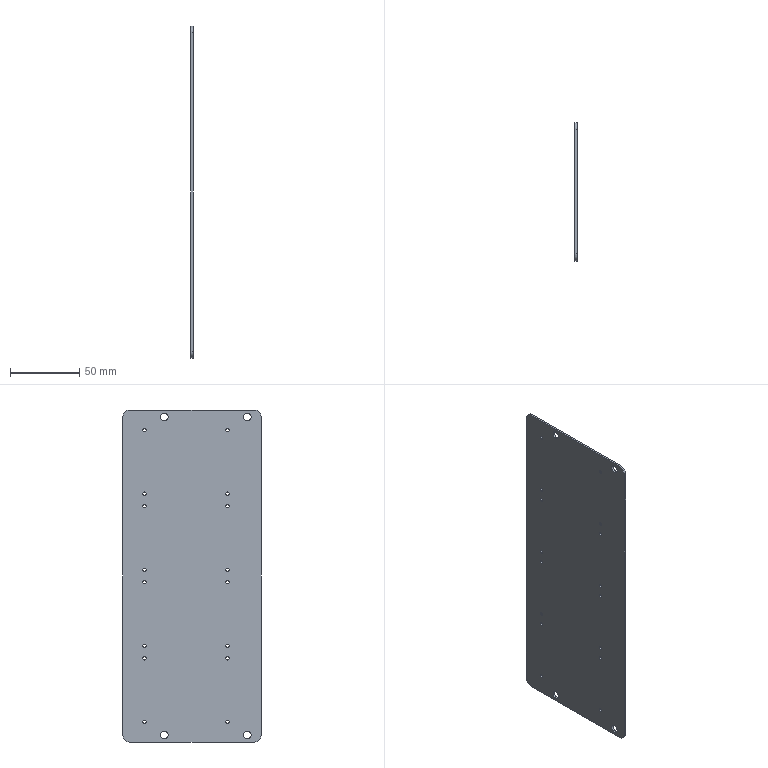Part | NX | features BREP 1 | 1 solid | 30 faces | box 1.5 x 100 x 240 mm | volume 35707 mm3 | cylinder 24 | plane 6 | commonest cylinder face diameters 2.5 x16 5.5 x4 10 x4
STEP:
#1=CARTESIAN_POINT('',(1.5,20.,-117.75));
#2=VERTEX_POINT('',#1);
#3=CARTESIAN_POINT('',(1.5,20.,-115.));
#4=DIRECTION('',(1.,0.,0.));
#5=DIRECTION('',(0.,0.,-1.));
#6=AXIS2_PLACEMENT_3D('',#3,#4,#5);
#7=CIRCLE('',#6,2.75);
#8=EDGE_CURVE('',#2,#2,#7,.T.);
#9=ORIENTED_EDGE('',*,*,#8,.T.);
#10=EDGE_LOOP('',(#9));
#11=FACE_BOUND('',#10,.T.);
#12=CARTESIAN_POINT('',(0.,20.,-117.75));
#13=VERTEX_POINT('',#12);
#14=CARTESIAN_POINT('',(0.,20.,-115.));
#15=DIRECTION('',(1.,0.,0.));
#16=DIRECTION('',(0.,0.,-1.));
#17=AXIS2_PLACEMENT_3D('',#14,#15,#16);
#18=CIRCLE('',#17,2.75);
#19=EDGE_CURVE('',#13,#13,#18,.T.);
#20=ORIENTED_EDGE('',*,*,#19,.F.);
#21=EDGE_LOOP('',(#20));
#22=FACE_BOUND('',#21,.T.);
#23=CARTESIAN_POINT('',(1.5,20.,-115.));
#24=DIRECTION('',(1.,0.,0.));
#25=DIRECTION('',(0.,0.,-1.));
#26=AXIS2_PLACEMENT_3D('',#23,#24,#25);
#27=CYLINDRICAL_SURFACE('',#26,2.75);
#28=ADVANCED_FACE('',(#11,#22),#27,.F.);
#29=CARTESIAN_POINT('',(1.5,-40.,-117.75));
#30=VERTEX_POINT('',#29);
#31=CARTESIAN_POINT('',(1.5,-40.,-115.));
#32=DIRECTION('',(1.,0.,0.));
#33=DIRECTION('',(0.,0.,-1.));
#34=AXIS2_PLACEMENT_3D('',#31,#32,#33);
#35=CIRCLE('',#34,2.75);
#36=EDGE_CURVE('',#30,#30,#35,.T.);
#37=ORIENTED_EDGE('',*,*,#36,.T.);
#38=EDGE_LOOP('',(#37));
#39=FACE_BOUND('',#38,.T.);
#40=CARTESIAN_POINT('',(0.,-40.,-117.75));
#41=VERTEX_POINT('',#40);
#42=CARTESIAN_POINT('',(0.,-40.,-115.));
#43=DIRECTION('',(1.,0.,0.));
#44=DIRECTION('',(0.,0.,-1.));
#45=AXIS2_PLACEMENT_3D('',#42,#43,#44);
#46=CIRCLE('',#45,2.75);
#47=EDGE_CURVE('',#41,#41,#46,.T.);
#48=ORIENTED_EDGE('',*,*,#47,.F.);
#49=EDGE_LOOP('',(#48));
#50=FACE_BOUND('',#49,.T.);
#51=CARTESIAN_POINT('',(1.5,-40.,-115.));
#52=DIRECTION('',(1.,0.,0.));
#53=DIRECTION('',(0.,0.,-1.));
#54=AXIS2_PLACEMENT_3D('',#51,#52,#53);
#55=CYLINDRICAL_SURFACE('',#54,2.75);
#56=ADVANCED_FACE('',(#39,#50),#55,.F.);
#57=CARTESIAN_POINT('',(1.5,20.,112.25));
#58=VERTEX_POINT('',#57);
#59=CARTESIAN_POINT('',(1.5,20.,115.));
#60=DIRECTION('',(1.,0.,0.));
#61=DIRECTION('',(0.,0.,-1.));
#62=AXIS2_PLACEMENT_3D('',#59,#60,#61);
#63=CIRCLE('',#62,2.75);
#64=EDGE_CURVE('',#58,#58,#63,.T.);
#65=ORIENTED_EDGE('',*,*,#64,.T.);
#66=EDGE_LOOP('',(#65));
#67=FACE_BOUND('',#66,.T.);
#68=CARTESIAN_POINT('',(0.,20.,112.25));
#69=VERTEX_POINT('',#68);
#70=CARTESIAN_POINT('',(0.,20.,115.));
#71=DIRECTION('',(1.,0.,0.));
#72=DIRECTION('',(0.,0.,-1.));
#73=AXIS2_PLACEMENT_3D('',#70,#71,#72);
#74=CIRCLE('',#73,2.75);
#75=EDGE_CURVE('',#69,#69,#74,.T.);
#76=ORIENTED_EDGE('',*,*,#75,.F.);
#77=EDGE_LOOP('',(#76));
#78=FACE_BOUND('',#77,.T.);
#79=CARTESIAN_POINT('',(1.5,20.,115.));
#80=DIRECTION('',(1.,0.,0.));
#81=DIRECTION('',(0.,0.,-1.));
#82=AXIS2_PLACEMENT_3D('',#79,#80,#81);
#83=CYLINDRICAL_SURFACE('',#82,2.75);
#84=ADVANCED_FACE('',(#67,#78),#83,.F.);
#85=CARTESIAN_POINT('',(1.5,-40.,112.25));
#86=VERTEX_POINT('',#85);
#87=CARTESIAN_POINT('',(1.5,-40.,115.));
#88=DIRECTION('',(1.,0.,0.));
#89=DIRECTION('',(0.,0.,-1.));
#90=AXIS2_PLACEMENT_3D('',#87,#88,#89);
#91=CIRCLE('',#90,2.75);
#92=EDGE_CURVE('',#86,#86,#91,.T.);
#93=ORIENTED_EDGE('',*,*,#92,.T.);
#94=EDGE_LOOP('',(#93));
#95=FACE_BOUND('',#94,.T.);
#96=CARTESIAN_POINT('',(0.,-40.,112.25));
#97=VERTEX_POINT('',#96);
#98=CARTESIAN_POINT('',(0.,-40.,115.));
#99=DIRECTION('',(1.,0.,0.));
#100=DIRECTION('',(0.,0.,-1.));
#101=AXIS2_PLACEMENT_3D('',#98,#99,#100);
#102=CIRCLE('',#101,2.75);
#103=EDGE_CURVE('',#97,#97,#102,.T.);
#104=ORIENTED_EDGE('',*,*,#103,.F.);
#105=EDGE_LOOP('',(#104));
#106=FACE_BOUND('',#105,.T.);
#107=CARTESIAN_POINT('',(1.5,-40.,115.));
#108=DIRECTION('',(1.,0.,0.));
#109=DIRECTION('',(0.,0.,-1.));
#110=AXIS2_PLACEMENT_3D('',#107,#108,#109);
#111=CYLINDRICAL_SURFACE('',#110,2.75);
#112=ADVANCED_FACE('',(#95,#106),#111,.F.);
#113=CARTESIAN_POINT('',(1.5,34.373,-106.75));
#114=VERTEX_POINT('',#113);
#115=CARTESIAN_POINT('',(1.5,34.373,-105.5));
#116=DIRECTION('',(1.,0.,0.));
#117=DIRECTION('',(0.,0.,-1.));
#118=AXIS2_PLACEMENT_3D('',#115,#116,#117);
#119=CIRCLE('',#118,1.25);
#120=EDGE_CURVE('',#114,#114,#119,.T.);
#121=ORIENTED_EDGE('',*,*,#120,.T.);
#122=EDGE_LOOP('',(#121));
#123=FACE_BOUND('',#122,.T.);
#124=CARTESIAN_POINT('',(0.,34.373,-106.75));
#125=VERTEX_POINT('',#124);
#126=CARTESIAN_POINT('',(0.,34.373,-105.5));
#127=DIRECTION('',(1.,0.,0.));
#128=DIRECTION('',(0.,0.,-1.));
#129=AXIS2_PLACEMENT_3D('',#126,#127,#128);
#130=CIRCLE('',#129,1.25);
#131=EDGE_CURVE('',#125,#125,#130,.T.);
#132=ORIENTED_EDGE('',*,*,#131,.F.);
#133=EDGE_LOOP('',(#132));
#134=FACE_BOUND('',#133,.T.);
#135=CARTESIAN_POINT('',(1.5,34.373,-105.5));
#136=DIRECTION('',(1.,0.,0.));
#137=DIRECTION('',(0.,0.,-1.));
#138=AXIS2_PLACEMENT_3D('',#135,#136,#137);
#139=CYLINDRICAL_SURFACE('',#138,1.25);
#140=ADVANCED_FACE('',(#123,#134),#139,.F.);
#141=CARTESIAN_POINT('',(1.5,34.373,-60.75));
#142=VERTEX_POINT('',#141);
#143=CARTESIAN_POINT('',(1.5,34.373,-59.5));
#144=DIRECTION('',(1.,0.,0.));
#145=DIRECTION('',(0.,0.,-1.));
#146=AXIS2_PLACEMENT_3D('',#143,#144,#145);
#147=CIRCLE('',#146,1.25);
#148=EDGE_CURVE('',#142,#142,#147,.T.);
#149=ORIENTED_EDGE('',*,*,#148,.T.);
#150=EDGE_LOOP('',(#149));
#151=FACE_BOUND('',#150,.T.);
#152=CARTESIAN_POINT('',(0.,34.373,-60.75));
#153=VERTEX_POINT('',#152);
#154=CARTESIAN_POINT('',(0.,34.373,-59.5));
#155=DIRECTION('',(1.,0.,0.));
#156=DIRECTION('',(0.,0.,-1.));
#157=AXIS2_PLACEMENT_3D('',#154,#155,#156);
#158=CIRCLE('',#157,1.25);
#159=EDGE_CURVE('',#153,#153,#158,.T.);
#160=ORIENTED_EDGE('',*,*,#159,.F.);
#161=EDGE_LOOP('',(#160));
#162=FACE_BOUND('',#161,.T.);
#163=CARTESIAN_POINT('',(1.5,34.373,-59.5));
#164=DIRECTION('',(1.,0.,0.));
#165=DIRECTION('',(0.,0.,-1.));
#166=AXIS2_PLACEMENT_3D('',#163,#164,#165);
#167=CYLINDRICAL_SURFACE('',#166,1.25);
#168=ADVANCED_FACE('',(#151,#162),#167,.F.);
#169=CARTESIAN_POINT('',(1.5,34.373,-51.75));
#170=VERTEX_POINT('',#169);
#171=CARTESIAN_POINT('',(1.5,34.373,-50.5));
#172=DIRECTION('',(1.,0.,0.));
#173=DIRECTION('',(0.,0.,-1.));
#174=AXIS2_PLACEMENT_3D('',#171,#172,#173);
#175=CIRCLE('',#174,1.25);
#176=EDGE_CURVE('',#170,#170,#175,.T.);
#177=ORIENTED_EDGE('',*,*,#176,.T.);
#178=EDGE_LOOP('',(#177));
#179=FACE_BOUND('',#178,.T.);
#180=CARTESIAN_POINT('',(0.,34.373,-51.75));
#181=VERTEX_POINT('',#180);
#182=CARTESIAN_POINT('',(0.,34.373,-50.5));
#183=DIRECTION('',(1.,0.,0.));
#184=DIRECTION('',(0.,0.,-1.));
#185=AXIS2_PLACEMENT_3D('',#182,#183,#184);
#186=CIRCLE('',#185,1.25);
#187=EDGE_CURVE('',#181,#181,#186,.T.);
#188=ORIENTED_EDGE('',*,*,#187,.F.);
#189=EDGE_LOOP('',(#188));
#190=FACE_BOUND('',#189,.T.);
#191=CARTESIAN_POINT('',(1.5,34.373,-50.5));
#192=DIRECTION('',(1.,0.,0.));
#193=DIRECTION('',(0.,0.,-1.));
#194=AXIS2_PLACEMENT_3D('',#191,#192,#193);
#195=CYLINDRICAL_SURFACE('',#194,1.25);
#196=ADVANCED_FACE('',(#179,#190),#195,.F.);
#197=CARTESIAN_POINT('',(1.5,34.373,-5.75));
#198=VERTEX_POINT('',#197);
#199=CARTESIAN_POINT('',(1.5,34.373,-4.5));
#200=DIRECTION('',(1.,0.,0.));
#201=DIRECTION('',(0.,0.,-1.));
#202=AXIS2_PLACEMENT_3D('',#199,#200,#201);
#203=CIRCLE('',#202,1.25);
#204=EDGE_CURVE('',#198,#198,#203,.T.);
#205=ORIENTED_EDGE('',*,*,#204,.T.);
#206=EDGE_LOOP('',(#205));
#207=FACE_BOUND('',#206,.T.);
#208=CARTESIAN_POINT('',(0.,34.373,-5.75));
#209=VERTEX_POINT('',#208);
#210=CARTESIAN_POINT('',(0.,34.373,-4.5));
#211=DIRECTION('',(1.,0.,0.));
#212=DIRECTION('',(0.,0.,-1.));
#213=AXIS2_PLACEMENT_3D('',#210,#211,#212);
#214=CIRCLE('',#213,1.25);
#215=EDGE_CURVE('',#209,#209,#214,.T.);
#216=ORIENTED_EDGE('',*,*,#215,.F.);
#217=EDGE_LOOP('',(#216));
#218=FACE_BOUND('',#217,.T.);
#219=CARTESIAN_POINT('',(1.5,34.373,-4.5));
#220=DIRECTION('',(1.,0.,0.));
#221=DIRECTION('',(0.,0.,-1.));
#222=AXIS2_PLACEMENT_3D('',#219,#220,#221);
#223=CYLINDRICAL_SURFACE('',#222,1.25);
#224=ADVANCED_FACE('',(#207,#218),#223,.F.);
#225=CARTESIAN_POINT('',(1.5,-25.627,-51.75));
#226=VERTEX_POINT('',#225);
#227=CARTESIAN_POINT('',(1.5,-25.627,-50.5));
#228=DIRECTION('',(1.,0.,0.));
#229=DIRECTION('',(0.,0.,-1.));
#230=AXIS2_PLACEMENT_3D('',#227,#228,#229);
#231=CIRCLE('',#230,1.25);
#232=EDGE_CURVE('',#226,#226,#231,.T.);
#233=ORIENTED_EDGE('',*,*,#232,.T.);
#234=EDGE_LOOP('',(#233));
#235=FACE_BOUND('',#234,.T.);
#236=CARTESIAN_POINT('',(0.,-25.627,-51.75));
#237=VERTEX_POINT('',#236);
#238=CARTESIAN_POINT('',(0.,-25.627,-50.5));
#239=DIRECTION('',(1.,0.,0.));
#240=DIRECTION('',(0.,0.,-1.));
#241=AXIS2_PLACEMENT_3D('',#238,#239,#240);
#242=CIRCLE('',#241,1.25);
#243=EDGE_CURVE('',#237,#237,#242,.T.);
#244=ORIENTED_EDGE('',*,*,#243,.F.);
#245=EDGE_LOOP('',(#244));
#246=FACE_BOUND('',#245,.T.);
#247=CARTESIAN_POINT('',(1.5,-25.627,-50.5));
#248=DIRECTION('',(1.,0.,0.));
#249=DIRECTION('',(0.,0.,-1.));
#250=AXIS2_PLACEMENT_3D('',#247,#248,#249);
#251=CYLINDRICAL_SURFACE('',#250,1.25);
#252=ADVANCED_FACE('',(#235,#246),#251,.F.);
#253=CARTESIAN_POINT('',(1.5,-25.627,-5.75));
#254=VERTEX_POINT('',#253);
#255=CARTESIAN_POINT('',(1.5,-25.627,-4.5));
#256=DIRECTION('',(1.,0.,0.));
#257=DIRECTION('',(0.,0.,-1.));
#258=AXIS2_PLACEMENT_3D('',#255,#256,#257);
#259=CIRCLE('',#258,1.25);
#260=EDGE_CURVE('',#254,#254,#259,.T.);
#261=ORIENTED_EDGE('',*,*,#260,.T.);
#262=EDGE_LOOP('',(#261));
#263=FACE_BOUND('',#262,.T.);
#264=CARTESIAN_POINT('',(0.,-25.627,-5.75));
#265=VERTEX_POINT('',#264);
#266=CARTESIAN_POINT('',(0.,-25.627,-4.5));
#267=DIRECTION('',(1.,0.,0.));
#268=DIRECTION('',(0.,0.,-1.));
#269=AXIS2_PLACEMENT_3D('',#266,#267,#268);
#270=CIRCLE('',#269,1.25);
#271=EDGE_CURVE('',#265,#265,#270,.T.);
#272=ORIENTED_EDGE('',*,*,#271,.F.);
#273=EDGE_LOOP('',(#272));
#274=FACE_BOUND('',#273,.T.);
#275=CARTESIAN_POINT('',(1.5,-25.627,-4.5));
#276=DIRECTION('',(1.,0.,0.));
#277=DIRECTION('',(0.,0.,-1.));
#278=AXIS2_PLACEMENT_3D('',#275,#276,#277);
#279=CYLINDRICAL_SURFACE('',#278,1.25);
#280=ADVANCED_FACE('',(#263,#274),#279,.F.);
#281=CARTESIAN_POINT('',(1.5,-25.627,-106.75));
#282=VERTEX_POINT('',#281);
#283=CARTESIAN_POINT('',(1.5,-25.627,-105.5));
#284=DIRECTION('',(1.,0.,0.));
#285=DIRECTION('',(0.,0.,-1.));
#286=AXIS2_PLACEMENT_3D('',#283,#284,#285);
#287=CIRCLE('',#286,1.25);
#288=EDGE_CURVE('',#282,#282,#287,.T.);
#289=ORIENTED_EDGE('',*,*,#288,.T.);
#290=EDGE_LOOP('',(#289));
#291=FACE_BOUND('',#290,.T.);
#292=CARTESIAN_POINT('',(0.,-25.627,-106.75));
#293=VERTEX_POINT('',#292);
#294=CARTESIAN_POINT('',(0.,-25.627,-105.5));
#295=DIRECTION('',(1.,0.,0.));
#296=DIRECTION('',(0.,0.,-1.));
#297=AXIS2_PLACEMENT_3D('',#294,#295,#296);
#298=CIRCLE('',#297,1.25);
#299=EDGE_CURVE('',#293,#293,#298,.T.);
#300=ORIENTED_EDGE('',*,*,#299,.F.);
#301=EDGE_LOOP('',(#300));
#302=FACE_BOUND('',#301,.T.);
#303=CARTESIAN_POINT('',(1.5,-25.627,-105.5));
#304=DIRECTION('',(1.,0.,0.));
#305=DIRECTION('',(0.,0.,-1.));
#306=AXIS2_PLACEMENT_3D('',#303,#304,#305);
#307=CYLINDRICAL_SURFACE('',#306,1.25);
#308=ADVANCED_FACE('',(#291,#302),#307,.F.);
#309=CARTESIAN_POINT('',(1.5,-25.627,-60.75));
#310=VERTEX_POINT('',#309);
#311=CARTESIAN_POINT('',(1.5,-25.627,-59.5));
#312=DIRECTION('',(1.,0.,0.));
#313=DIRECTION('',(0.,0.,-1.));
#314=AXIS2_PLACEMENT_3D('',#311,#312,#313);
#315=CIRCLE('',#314,1.25);
#316=EDGE_CURVE('',#310,#310,#315,.T.);
#317=ORIENTED_EDGE('',*,*,#316,.T.);
#318=EDGE_LOOP('',(#317));
#319=FACE_BOUND('',#318,.T.);
#320=CARTESIAN_POINT('',(0.,-25.627,-60.75));
#321=VERTEX_POINT('',#320);
#322=CARTESIAN_POINT('',(0.,-25.627,-59.5));
#323=DIRECTION('',(1.,0.,0.));
#324=DIRECTION('',(0.,0.,-1.));
#325=AXIS2_PLACEMENT_3D('',#322,#323,#324);
#326=CIRCLE('',#325,1.25);
#327=EDGE_CURVE('',#321,#321,#326,.T.);
#328=ORIENTED_EDGE('',*,*,#327,.F.);
#329=EDGE_LOOP('',(#328));
#330=FACE_BOUND('',#329,.T.);
#331=CARTESIAN_POINT('',(1.5,-25.627,-59.5));
#332=DIRECTION('',(1.,0.,0.));
#333=DIRECTION('',(0.,0.,-1.));
#334=AXIS2_PLACEMENT_3D('',#331,#332,#333);
#335=CYLINDRICAL_SURFACE('',#334,1.25);
#336=ADVANCED_FACE('',(#319,#330),#335,.F.);
#337=CARTESIAN_POINT('',(1.5,-25.627,3.25));
#338=VERTEX_POINT('',#337);
#339=CARTESIAN_POINT('',(1.5,-25.627,4.5));
#340=DIRECTION('',(1.,0.,0.));
#341=DIRECTION('',(0.,0.,-1.));
#342=AXIS2_PLACEMENT_3D('',#339,#340,#341);
#343=CIRCLE('',#342,1.25);
#344=EDGE_CURVE('',#338,#338,#343,.T.);
#345=ORIENTED_EDGE('',*,*,#344,.T.);
#346=EDGE_LOOP('',(#345));
#347=FACE_BOUND('',#346,.T.);
#348=CARTESIAN_POINT('',(0.,-25.627,3.25));
#349=VERTEX_POINT('',#348);
#350=CARTESIAN_POINT('',(0.,-25.627,4.5));
#351=DIRECTION('',(1.,0.,0.));
#352=DIRECTION('',(0.,0.,-1.));
#353=AXIS2_PLACEMENT_3D('',#350,#351,#352);
#354=CIRCLE('',#353,1.25);
#355=EDGE_CURVE('',#349,#349,#354,.T.);
#356=ORIENTED_EDGE('',*,*,#355,.F.);
#357=EDGE_LOOP('',(#356));
#358=FACE_BOUND('',#357,.T.);
#359=CARTESIAN_POINT('',(1.5,-25.627,4.5));
#360=DIRECTION('',(1.,0.,0.));
#361=DIRECTION('',(0.,0.,-1.));
#362=AXIS2_PLACEMENT_3D('',#359,#360,#361);
#363=CYLINDRICAL_SURFACE('',#362,1.25);
#364=ADVANCED_FACE('',(#347,#358),#363,.F.);
#365=CARTESIAN_POINT('',(1.5,-25.627,49.25));
#366=VERTEX_POINT('',#365);
#367=CARTESIAN_POINT('',(1.5,-25.627,50.5));
#368=DIRECTION('',(1.,0.,0.));
#369=DIRECTION('',(0.,0.,-1.));
#370=AXIS2_PLACEMENT_3D('',#367,#368,#369);
#371=CIRCLE('',#370,1.25);
#372=EDGE_CURVE('',#366,#366,#371,.T.);
#373=ORIENTED_EDGE('',*,*,#372,.T.);
#374=EDGE_LOOP('',(#373));
#375=FACE_BOUND('',#374,.T.);
#376=CARTESIAN_POINT('',(0.,-25.627,49.25));
#377=VERTEX_POINT('',#376);
#378=CARTESIAN_POINT('',(0.,-25.627,50.5));
#379=DIRECTION('',(1.,0.,0.));
#380=DIRECTION('',(0.,0.,-1.));
#381=AXIS2_PLACEMENT_3D('',#378,#379,#380);
#382=CIRCLE('',#381,1.25);
#383=EDGE_CURVE('',#377,#377,#382,.T.);
#384=ORIENTED_EDGE('',*,*,#383,.F.);
#385=EDGE_LOOP('',(#384));
#386=FACE_BOUND('',#385,.T.);
#387=CARTESIAN_POINT('',(1.5,-25.627,50.5));
#388=DIRECTION('',(1.,0.,0.));
#389=DIRECTION('',(0.,0.,-1.));
#390=AXIS2_PLACEMENT_3D('',#387,#388,#389);
#391=CYLINDRICAL_SURFACE('',#390,1.25);
#392=ADVANCED_FACE('',(#375,#386),#391,.F.);
#393=CARTESIAN_POINT('',(1.5,34.373,3.25));
#394=VERTEX_POINT('',#393);
#395=CARTESIAN_POINT('',(1.5,34.373,4.5));
#396=DIRECTION('',(1.,0.,0.));
#397=DIRECTION('',(0.,0.,-1.));
#398=AXIS2_PLACEMENT_3D('',#395,#396,#397);
#399=CIRCLE('',#398,1.25);
#400=EDGE_CURVE('',#394,#394,#399,.T.);
#401=ORIENTED_EDGE('',*,*,#400,.T.);
#402=EDGE_LOOP('',(#401));
#403=FACE_BOUND('',#402,.T.);
#404=CARTESIAN_POINT('',(0.,34.373,3.25));
#405=VERTEX_POINT('',#404);
#406=CARTESIAN_POINT('',(0.,34.373,4.5));
#407=DIRECTION('',(1.,0.,0.));
#408=DIRECTION('',(0.,0.,-1.));
#409=AXIS2_PLACEMENT_3D('',#406,#407,#408);
#410=CIRCLE('',#409,1.25);
#411=EDGE_CURVE('',#405,#405,#410,.T.);
#412=ORIENTED_EDGE('',*,*,#411,.F.);
#413=EDGE_LOOP('',(#412));
#414=FACE_BOUND('',#413,.T.);
#415=CARTESIAN_POINT('',(1.5,34.373,4.5));
#416=DIRECTION('',(1.,0.,0.));
#417=DIRECTION('',(0.,0.,-1.));
#418=AXIS2_PLACEMENT_3D('',#415,#416,#417);
#419=CYLINDRICAL_SURFACE('',#418,1.25);
#420=ADVANCED_FACE('',(#403,#414),#419,.F.);
#421=CARTESIAN_POINT('',(1.5,34.373,49.25));
#422=VERTEX_POINT('',#421);
#423=CARTESIAN_POINT('',(1.5,34.373,50.5));
#424=DIRECTION('',(1.,0.,0.));
#425=DIRECTION('',(0.,0.,-1.));
#426=AXIS2_PLACEMENT_3D('',#423,#424,#425);
#427=CIRCLE('',#426,1.25);
#428=EDGE_CURVE('',#422,#422,#427,.T.);
#429=ORIENTED_EDGE('',*,*,#428,.T.);
#430=EDGE_LOOP('',(#429));
#431=FACE_BOUND('',#430,.T.);
#432=CARTESIAN_POINT('',(0.,34.373,49.25));
#433=VERTEX_POINT('',#432);
#434=CARTESIAN_POINT('',(0.,34.373,50.5));
#435=DIRECTION('',(1.,0.,0.));
#436=DIRECTION('',(0.,0.,-1.));
#437=AXIS2_PLACEMENT_3D('',#434,#435,#436);
#438=CIRCLE('',#437,1.25);
#439=EDGE_CURVE('',#433,#433,#438,.T.);
#440=ORIENTED_EDGE('',*,*,#439,.F.);
#441=EDGE_LOOP('',(#440));
#442=FACE_BOUND('',#441,.T.);
#443=CARTESIAN_POINT('',(1.5,34.373,50.5));
#444=DIRECTION('',(1.,0.,0.));
#445=DIRECTION('',(0.,0.,-1.));
#446=AXIS2_PLACEMENT_3D('',#443,#444,#445);
#447=CYLINDRICAL_SURFACE('',#446,1.25);
#448=ADVANCED_FACE('',(#431,#442),#447,.F.);
#449=CARTESIAN_POINT('',(1.5,34.373,58.25));
#450=VERTEX_POINT('',#449);
#451=CARTESIAN_POINT('',(1.5,34.373,59.5));
#452=DIRECTION('',(1.,0.,0.));
#453=DIRECTION('',(0.,0.,-1.));
#454=AXIS2_PLACEMENT_3D('',#451,#452,#453);
#455=CIRCLE('',#454,1.25);
#456=EDGE_CURVE('',#450,#450,#455,.T.);
#457=ORIENTED_EDGE('',*,*,#456,.T.);
#458=EDGE_LOOP('',(#457));
#459=FACE_BOUND('',#458,.T.);
#460=CARTESIAN_POINT('',(0.,34.373,58.25));
#461=VERTEX_POINT('',#460);
#462=CARTESIAN_POINT('',(0.,34.373,59.5));
#463=DIRECTION('',(1.,0.,0.));
#464=DIRECTION('',(0.,0.,-1.));
#465=AXIS2_PLACEMENT_3D('',#462,#463,#464);
#466=CIRCLE('',#465,1.25);
#467=EDGE_CURVE('',#461,#461,#466,.T.);
#468=ORIENTED_EDGE('',*,*,#467,.F.);
#469=EDGE_LOOP('',(#468));
#470=FACE_BOUND('',#469,.T.);
#471=CARTESIAN_POINT('',(1.5,34.373,59.5));
#472=DIRECTION('',(1.,0.,0.));
#473=DIRECTION('',(0.,0.,-1.));
#474=AXIS2_PLACEMENT_3D('',#471,#472,#473);
#475=CYLINDRICAL_SURFACE('',#474,1.25);
#476=ADVANCED_FACE('',(#459,#470),#475,.F.);
#477=CARTESIAN_POINT('',(1.5,34.373,104.25));
#478=VERTEX_POINT('',#477);
#479=CARTESIAN_POINT('',(1.5,34.373,105.5));
#480=DIRECTION('',(1.,0.,0.));
#481=DIRECTION('',(0.,0.,-1.));
#482=AXIS2_PLACEMENT_3D('',#479,#480,#481);
#483=CIRCLE('',#482,1.25);
#484=EDGE_CURVE('',#478,#478,#483,.T.);
#485=ORIENTED_EDGE('',*,*,#484,.T.);
#486=EDGE_LOOP('',(#485));
#487=FACE_BOUND('',#486,.T.);
#488=CARTESIAN_POINT('',(0.,34.373,104.25));
#489=VERTEX_POINT('',#488);
#490=CARTESIAN_POINT('',(0.,34.373,105.5));
#491=DIRECTION('',(1.,0.,0.));
#492=DIRECTION('',(0.,0.,-1.));
#493=AXIS2_PLACEMENT_3D('',#490,#491,#492);
#494=CIRCLE('',#493,1.25);
#495=EDGE_CURVE('',#489,#489,#494,.T.);
#496=ORIENTED_EDGE('',*,*,#495,.F.);
#497=EDGE_LOOP('',(#496));
#498=FACE_BOUND('',#497,.T.);
#499=CARTESIAN_POINT('',(1.5,34.373,105.5));
#500=DIRECTION('',(1.,0.,0.));
#501=DIRECTION('',(0.,0.,-1.));
#502=AXIS2_PLACEMENT_3D('',#499,#500,#501);
#503=CYLINDRICAL_SURFACE('',#502,1.25);
#504=ADVANCED_FACE('',(#487,#498),#503,.F.);
#505=CARTESIAN_POINT('',(1.5,-25.627,58.25));
#506=VERTEX_POINT('',#505);
#507=CARTESIAN_POINT('',(1.5,-25.627,59.5));
#508=DIRECTION('',(1.,0.,0.));
#509=DIRECTION('',(0.,0.,-1.));
#510=AXIS2_PLACEMENT_3D('',#507,#508,#509);
#511=CIRCLE('',#510,1.25);
#512=EDGE_CURVE('',#506,#506,#511,.T.);
#513=ORIENTED_EDGE('',*,*,#512,.T.);
#514=EDGE_LOOP('',(#513));
#515=FACE_BOUND('',#514,.T.);
#516=CARTESIAN_POINT('',(0.,-25.627,58.25));
#517=VERTEX_POINT('',#516);
#518=CARTESIAN_POINT('',(0.,-25.627,59.5));
#519=DIRECTION('',(1.,0.,0.));
#520=DIRECTION('',(0.,0.,-1.));
#521=AXIS2_PLACEMENT_3D('',#518,#519,#520);
#522=CIRCLE('',#521,1.25);
#523=EDGE_CURVE('',#517,#517,#522,.T.);
#524=ORIENTED_EDGE('',*,*,#523,.F.);
#525=EDGE_LOOP('',(#524));
#526=FACE_BOUND('',#525,.T.);
#527=CARTESIAN_POINT('',(1.5,-25.627,59.5));
#528=DIRECTION('',(1.,0.,0.));
#529=DIRECTION('',(0.,0.,-1.));
#530=AXIS2_PLACEMENT_3D('',#527,#528,#529);
#531=CYLINDRICAL_SURFACE('',#530,1.25);
#532=ADVANCED_FACE('',(#515,#526),#531,.F.);
#533=CARTESIAN_POINT('',(1.5,-25.627,104.25));
#534=VERTEX_POINT('',#533);
#535=CARTESIAN_POINT('',(1.5,-25.627,105.5));
#536=DIRECTION('',(1.,0.,0.));
#537=DIRECTION('',(0.,0.,-1.));
#538=AXIS2_PLACEMENT_3D('',#535,#536,#537);
#539=CIRCLE('',#538,1.25);
#540=EDGE_CURVE('',#534,#534,#539,.T.);
#541=ORIENTED_EDGE('',*,*,#540,.T.);
#542=EDGE_LOOP('',(#541));
#543=FACE_BOUND('',#542,.T.);
#544=CARTESIAN_POINT('',(0.,-25.627,104.25));
#545=VERTEX_POINT('',#544);
#546=CARTESIAN_POINT('',(0.,-25.627,105.5));
#547=DIRECTION('',(1.,0.,0.));
#548=DIRECTION('',(0.,0.,-1.));
#549=AXIS2_PLACEMENT_3D('',#546,#547,#548);
#550=CIRCLE('',#549,1.25);
#551=EDGE_CURVE('',#545,#545,#550,.T.);
#552=ORIENTED_EDGE('',*,*,#551,.F.);
#553=EDGE_LOOP('',(#552));
#554=FACE_BOUND('',#553,.T.);
#555=CARTESIAN_POINT('',(1.5,-25.627,105.5));
#556=DIRECTION('',(1.,0.,0.));
#557=DIRECTION('',(0.,0.,-1.));
#558=AXIS2_PLACEMENT_3D('',#555,#556,#557);
#559=CYLINDRICAL_SURFACE('',#558,1.25);
#560=ADVANCED_FACE('',(#543,#554),#559,.F.);
#561=CARTESIAN_POINT('',(0.,-45.,-120.));
#562=VERTEX_POINT('',#561);
#563=CARTESIAN_POINT('',(0.,45.,-120.));
#564=VERTEX_POINT('',#563);
#565=CARTESIAN_POINT('',(0.,50.,-120.));
#566=DIRECTION('',(0.,1.,0.));
#567=VECTOR('',#566,1000.);
#568=LINE('',#565,#567);
#569=EDGE_CURVE('',#562,#564,#568,.T.);
#570=ORIENTED_EDGE('',*,*,#569,.T.);
#571=CARTESIAN_POINT('',(1.5,45.,-120.));
#572=VERTEX_POINT('',#571);
#573=CARTESIAN_POINT('',(1.5,45.,-120.));
#574=DIRECTION('',(1.,0.,0.));
#575=VECTOR('',#574,1000.);
#576=LINE('',#573,#575);
#577=EDGE_CURVE('',#564,#572,#576,.T.);
#578=ORIENTED_EDGE('',*,*,#577,.T.);
#579=CARTESIAN_POINT('',(1.5,-45.,-120.));
#580=VERTEX_POINT('',#579);
#581=CARTESIAN_POINT('',(1.5,50.,-120.));
#582=DIRECTION('',(0.,1.,0.));
#583=VECTOR('',#582,1000.);
#584=LINE('',#581,#583);
#585=EDGE_CURVE('',#580,#572,#584,.T.);
#586=ORIENTED_EDGE('',*,*,#585,.F.);
#587=CARTESIAN_POINT('',(1.5,-45.,-120.));
#588=DIRECTION('',(-1.,0.,0.));
#589=VECTOR('',#588,1000.);
#590=LINE('',#587,#589);
#591=EDGE_CURVE('',#580,#562,#590,.T.);
#592=ORIENTED_EDGE('',*,*,#591,.T.);
#593=EDGE_LOOP('',(#570,#578,#586,#592));
#594=FACE_BOUND('',#593,.T.);
#595=CARTESIAN_POINT('',(1.5,50.,-120.));
#596=DIRECTION('',(0.,0.,1.));
#597=DIRECTION('',(0.,-1.,0.));
#598=AXIS2_PLACEMENT_3D('',#595,#596,#597);
#599=PLANE('',#598);
#600=ADVANCED_FACE('',(#594),#599,.F.);
#601=CARTESIAN_POINT('',(1.5,50.,-115.));
#602=VERTEX_POINT('',#601);
#603=CARTESIAN_POINT('',(1.5,50.,115.));
#604=VERTEX_POINT('',#603);
#605=CARTESIAN_POINT('',(1.5,50.,120.));
#606=DIRECTION('',(0.,0.,1.));
#607=VECTOR('',#606,1000.);
#608=LINE('',#605,#607);
#609=EDGE_CURVE('',#602,#604,#608,.T.);
#610=ORIENTED_EDGE('',*,*,#609,.F.);
#611=CARTESIAN_POINT('',(0.,50.,-115.));
#612=VERTEX_POINT('',#611);
#613=CARTESIAN_POINT('',(1.5,50.,-115.));
#614=DIRECTION('',(-1.,0.,0.));
#615=VECTOR('',#614,1000.);
#616=LINE('',#613,#615);
#617=EDGE_CURVE('',#602,#612,#616,.T.);
#618=ORIENTED_EDGE('',*,*,#617,.T.);
#619=CARTESIAN_POINT('',(0.,50.,115.));
#620=VERTEX_POINT('',#619);
#621=CARTESIAN_POINT('',(0.,50.,120.));
#622=DIRECTION('',(0.,0.,1.));
#623=VECTOR('',#622,1000.);
#624=LINE('',#621,#623);
#625=EDGE_CURVE('',#612,#620,#624,.T.);
#626=ORIENTED_EDGE('',*,*,#625,.T.);
#627=CARTESIAN_POINT('',(1.5,50.,115.));
#628=DIRECTION('',(1.,0.,0.));
#629=VECTOR('',#628,1000.);
#630=LINE('',#627,#629);
#631=EDGE_CURVE('',#620,#604,#630,.T.);
#632=ORIENTED_EDGE('',*,*,#631,.T.);
#633=EDGE_LOOP('',(#610,#618,#626,#632));
#634=FACE_BOUND('',#633,.T.);
#635=CARTESIAN_POINT('',(1.5,50.,120.));
#636=DIRECTION('',(0.,-1.,0.));
#637=DIRECTION('',(0.,0.,-1.));
#638=AXIS2_PLACEMENT_3D('',#635,#636,#637);
#639=PLANE('',#638);
#640=ADVANCED_FACE('',(#634),#639,.F.);
#641=CARTESIAN_POINT('',(0.,45.,120.));
#642=VERTEX_POINT('',#641);
#643=CARTESIAN_POINT('',(0.,-45.,120.));
#644=VERTEX_POINT('',#643);
#645=CARTESIAN_POINT('',(0.,50.,120.));
#646=DIRECTION('',(0.,-1.,0.));
#647=VECTOR('',#646,1000.);
#648=LINE('',#645,#647);
#649=EDGE_CURVE('',#642,#644,#648,.T.);
#650=ORIENTED_EDGE('',*,*,#649,.T.);
#651=CARTESIAN_POINT('',(1.5,-45.,120.));
#652=VERTEX_POINT('',#651);
#653=CARTESIAN_POINT('',(1.5,-45.,120.));
#654=DIRECTION('',(1.,0.,0.));
#655=VECTOR('',#654,1000.);
#656=LINE('',#653,#655);
#657=EDGE_CURVE('',#644,#652,#656,.T.);
#658=ORIENTED_EDGE('',*,*,#657,.T.);
#659=CARTESIAN_POINT('',(1.5,45.,120.));
#660=VERTEX_POINT('',#659);
#661=CARTESIAN_POINT('',(1.5,50.,120.));
#662=DIRECTION('',(0.,-1.,0.));
#663=VECTOR('',#662,1000.);
#664=LINE('',#661,#663);
#665=EDGE_CURVE('',#660,#652,#664,.T.);
#666=ORIENTED_EDGE('',*,*,#665,.F.);
#667=CARTESIAN_POINT('',(1.5,45.,120.));
#668=DIRECTION('',(-1.,0.,0.));
#669=VECTOR('',#668,1000.);
#670=LINE('',#667,#669);
#671=EDGE_CURVE('',#660,#642,#670,.T.);
#672=ORIENTED_EDGE('',*,*,#671,.T.);
#673=EDGE_LOOP('',(#650,#658,#666,#672));
#674=FACE_BOUND('',#673,.T.);
#675=CARTESIAN_POINT('',(1.5,50.,120.));
#676=DIRECTION('',(0.,0.,-1.));
#677=DIRECTION('',(0.,1.,0.));
#678=AXIS2_PLACEMENT_3D('',#675,#676,#677);
#679=PLANE('',#678);
#680=ADVANCED_FACE('',(#674),#679,.F.);
#681=CARTESIAN_POINT('',(0.,-50.,115.));
#682=VERTEX_POINT('',#681);
#683=CARTESIAN_POINT('',(0.,-50.,-115.));
#684=VERTEX_POINT('',#683);
#685=CARTESIAN_POINT('',(0.,-50.,120.));
#686=DIRECTION('',(0.,0.,-1.));
#687=VECTOR('',#686,1000.);
#688=LINE('',#685,#687);
#689=EDGE_CURVE('',#682,#684,#688,.T.);
#690=ORIENTED_EDGE('',*,*,#689,.T.);
#691=CARTESIAN_POINT('',(1.5,-50.,-115.));
#692=VERTEX_POINT('',#691);
#693=CARTESIAN_POINT('',(1.5,-50.,-115.));
#694=DIRECTION('',(1.,0.,0.));
#695=VECTOR('',#694,1000.);
#696=LINE('',#693,#695);
#697=EDGE_CURVE('',#684,#692,#696,.T.);
#698=ORIENTED_EDGE('',*,*,#697,.T.);
#699=CARTESIAN_POINT('',(1.5,-50.,115.));
#700=VERTEX_POINT('',#699);
#701=CARTESIAN_POINT('',(1.5,-50.,120.));
#702=DIRECTION('',(0.,0.,-1.));
#703=VECTOR('',#702,1000.);
#704=LINE('',#701,#703);
#705=EDGE_CURVE('',#700,#692,#704,.T.);
#706=ORIENTED_EDGE('',*,*,#705,.F.);
#707=CARTESIAN_POINT('',(1.5,-50.,115.));
#708=DIRECTION('',(-1.,0.,0.));
#709=VECTOR('',#708,1000.);
#710=LINE('',#707,#709);
#711=EDGE_CURVE('',#700,#682,#710,.T.);
#712=ORIENTED_EDGE('',*,*,#711,.T.);
#713=EDGE_LOOP('',(#690,#698,#706,#712));
#714=FACE_BOUND('',#713,.T.);
#715=CARTESIAN_POINT('',(1.5,-50.,120.));
#716=DIRECTION('',(0.,1.,0.));
#717=DIRECTION('',(0.,0.,1.));
#718=AXIS2_PLACEMENT_3D('',#715,#716,#717);
#719=PLANE('',#718);
#720=ADVANCED_FACE('',(#714),#719,.F.);
#721=ORIENTED_EDGE('',*,*,#8,.F.);
#722=EDGE_LOOP('',(#721));
#723=FACE_BOUND('',#722,.T.);
#724=ORIENTED_EDGE('',*,*,#36,.F.);
#725=EDGE_LOOP('',(#724));
#726=FACE_BOUND('',#725,.T.);
#727=ORIENTED_EDGE('',*,*,#64,.F.);
#728=EDGE_LOOP('',(#727));
#729=FACE_BOUND('',#728,.T.);
#730=ORIENTED_EDGE('',*,*,#92,.F.);
#731=EDGE_LOOP('',(#730));
#732=FACE_BOUND('',#731,.T.);
#733=ORIENTED_EDGE('',*,*,#120,.F.);
#734=EDGE_LOOP('',(#733));
#735=FACE_BOUND('',#734,.T.);
#736=ORIENTED_EDGE('',*,*,#148,.F.);
#737=EDGE_LOOP('',(#736));
#738=FACE_BOUND('',#737,.T.);
#739=ORIENTED_EDGE('',*,*,#176,.F.);
#740=EDGE_LOOP('',(#739));
#741=FACE_BOUND('',#740,.T.);
#742=ORIENTED_EDGE('',*,*,#204,.F.);
#743=EDGE_LOOP('',(#742));
#744=FACE_BOUND('',#743,.T.);
#745=ORIENTED_EDGE('',*,*,#232,.F.);
#746=EDGE_LOOP('',(#745));
#747=FACE_BOUND('',#746,.T.);
#748=ORIENTED_EDGE('',*,*,#260,.F.);
#749=EDGE_LOOP('',(#748));
#750=FACE_BOUND('',#749,.T.);
#751=ORIENTED_EDGE('',*,*,#288,.F.);
#752=EDGE_LOOP('',(#751));
#753=FACE_BOUND('',#752,.T.);
#754=ORIENTED_EDGE('',*,*,#316,.F.);
#755=EDGE_LOOP('',(#754));
#756=FACE_BOUND('',#755,.T.);
#757=ORIENTED_EDGE('',*,*,#344,.F.);
#758=EDGE_LOOP('',(#757));
#759=FACE_BOUND('',#758,.T.);
#760=ORIENTED_EDGE('',*,*,#372,.F.);
#761=EDGE_LOOP('',(#760));
#762=FACE_BOUND('',#761,.T.);
#763=ORIENTED_EDGE('',*,*,#400,.F.);
#764=EDGE_LOOP('',(#763));
#765=FACE_BOUND('',#764,.T.);
#766=ORIENTED_EDGE('',*,*,#428,.F.);
#767=EDGE_LOOP('',(#766));
#768=FACE_BOUND('',#767,.T.);
#769=ORIENTED_EDGE('',*,*,#456,.F.);
#770=EDGE_LOOP('',(#769));
#771=FACE_BOUND('',#770,.T.);
#772=ORIENTED_EDGE('',*,*,#484,.F.);
#773=EDGE_LOOP('',(#772));
#774=FACE_BOUND('',#773,.T.);
#775=ORIENTED_EDGE('',*,*,#512,.F.);
#776=EDGE_LOOP('',(#775));
#777=FACE_BOUND('',#776,.T.);
#778=ORIENTED_EDGE('',*,*,#540,.F.);
#779=EDGE_LOOP('',(#778));
#780=FACE_BOUND('',#779,.T.);
#781=ORIENTED_EDGE('',*,*,#585,.T.);
#782=CARTESIAN_POINT('',(1.5,45.,-115.));
#783=DIRECTION('',(1.,0.,0.));
#784=DIRECTION('',(0.,0.,-1.));
#785=AXIS2_PLACEMENT_3D('',#782,#783,#784);
#786=CIRCLE('',#785,5.);
#787=EDGE_CURVE('',#572,#602,#786,.T.);
#788=ORIENTED_EDGE('',*,*,#787,.T.);
#789=ORIENTED_EDGE('',*,*,#609,.T.);
#790=CARTESIAN_POINT('',(1.5,45.,115.));
#791=DIRECTION('',(1.,0.,0.));
#792=DIRECTION('',(0.,0.,-1.));
#793=AXIS2_PLACEMENT_3D('',#790,#791,#792);
#794=CIRCLE('',#793,5.);
#795=EDGE_CURVE('',#604,#660,#794,.T.);
#796=ORIENTED_EDGE('',*,*,#795,.T.);
#797=ORIENTED_EDGE('',*,*,#665,.T.);
#798=CARTESIAN_POINT('',(1.5,-45.,115.));
#799=DIRECTION('',(1.,0.,0.));
#800=DIRECTION('',(0.,0.,-1.));
#801=AXIS2_PLACEMENT_3D('',#798,#799,#800);
#802=CIRCLE('',#801,5.);
#803=EDGE_CURVE('',#652,#700,#802,.T.);
#804=ORIENTED_EDGE('',*,*,#803,.T.);
#805=ORIENTED_EDGE('',*,*,#705,.T.);
#806=CARTESIAN_POINT('',(1.5,-45.,-115.));
#807=DIRECTION('',(1.,0.,0.));
#808=DIRECTION('',(0.,0.,-1.));
#809=AXIS2_PLACEMENT_3D('',#806,#807,#808);
#810=CIRCLE('',#809,5.);
#811=EDGE_CURVE('',#692,#580,#810,.T.);
#812=ORIENTED_EDGE('',*,*,#811,.T.);
#813=EDGE_LOOP('',(#781,#788,#789,#796,#797,#804,#805,#812));
#814=FACE_BOUND('',#813,.T.);
#815=CARTESIAN_POINT('',(1.5,0.,0.));
#816=DIRECTION('',(1.,0.,0.));
#817=DIRECTION('',(0.,0.,-1.));
#818=AXIS2_PLACEMENT_3D('',#815,#816,#817);
#819=PLANE('',#818);
#820=ADVANCED_FACE('',(#723,#726,#729,#732,#735,#738,#741,#744,#747,#750,#753,#756,#759,#762,#765,#768,#771,#774,#777,#780,#814),#819,.T.);
#821=ORIENTED_EDGE('',*,*,#19,.T.);
#822=EDGE_LOOP('',(#821));
#823=FACE_BOUND('',#822,.T.);
#824=ORIENTED_EDGE('',*,*,#47,.T.);
#825=EDGE_LOOP('',(#824));
#826=FACE_BOUND('',#825,.T.);
#827=ORIENTED_EDGE('',*,*,#75,.T.);
#828=EDGE_LOOP('',(#827));
#829=FACE_BOUND('',#828,.T.);
#830=ORIENTED_EDGE('',*,*,#103,.T.);
#831=EDGE_LOOP('',(#830));
#832=FACE_BOUND('',#831,.T.);
#833=ORIENTED_EDGE('',*,*,#131,.T.);
#834=EDGE_LOOP('',(#833));
#835=FACE_BOUND('',#834,.T.);
#836=ORIENTED_EDGE('',*,*,#159,.T.);
#837=EDGE_LOOP('',(#836));
#838=FACE_BOUND('',#837,.T.);
#839=ORIENTED_EDGE('',*,*,#187,.T.);
#840=EDGE_LOOP('',(#839));
#841=FACE_BOUND('',#840,.T.);
#842=ORIENTED_EDGE('',*,*,#215,.T.);
#843=EDGE_LOOP('',(#842));
#844=FACE_BOUND('',#843,.T.);
#845=ORIENTED_EDGE('',*,*,#243,.T.);
#846=EDGE_LOOP('',(#845));
#847=FACE_BOUND('',#846,.T.);
#848=ORIENTED_EDGE('',*,*,#271,.T.);
#849=EDGE_LOOP('',(#848));
#850=FACE_BOUND('',#849,.T.);
#851=ORIENTED_EDGE('',*,*,#299,.T.);
#852=EDGE_LOOP('',(#851));
#853=FACE_BOUND('',#852,.T.);
#854=ORIENTED_EDGE('',*,*,#327,.T.);
#855=EDGE_LOOP('',(#854));
#856=FACE_BOUND('',#855,.T.);
#857=ORIENTED_EDGE('',*,*,#355,.T.);
#858=EDGE_LOOP('',(#857));
#859=FACE_BOUND('',#858,.T.);
#860=ORIENTED_EDGE('',*,*,#383,.T.);
#861=EDGE_LOOP('',(#860));
#862=FACE_BOUND('',#861,.T.);
#863=ORIENTED_EDGE('',*,*,#411,.T.);
#864=EDGE_LOOP('',(#863));
#865=FACE_BOUND('',#864,.T.);
#866=ORIENTED_EDGE('',*,*,#439,.T.);
#867=EDGE_LOOP('',(#866));
#868=FACE_BOUND('',#867,.T.);
#869=ORIENTED_EDGE('',*,*,#467,.T.);
#870=EDGE_LOOP('',(#869));
#871=FACE_BOUND('',#870,.T.);
#872=ORIENTED_EDGE('',*,*,#495,.T.);
#873=EDGE_LOOP('',(#872));
#874=FACE_BOUND('',#873,.T.);
#875=ORIENTED_EDGE('',*,*,#523,.T.);
#876=EDGE_LOOP('',(#875));
#877=FACE_BOUND('',#876,.T.);
#878=ORIENTED_EDGE('',*,*,#551,.T.);
#879=EDGE_LOOP('',(#878));
#880=FACE_BOUND('',#879,.T.);
#881=ORIENTED_EDGE('',*,*,#625,.F.);
#882=CARTESIAN_POINT('',(0.,45.,-115.));
#883=DIRECTION('',(-1.,0.,0.));
#884=DIRECTION('',(0.,0.,-1.));
#885=AXIS2_PLACEMENT_3D('',#882,#883,#884);
#886=CIRCLE('',#885,5.);
#887=EDGE_CURVE('',#612,#564,#886,.T.);
#888=ORIENTED_EDGE('',*,*,#887,.T.);
#889=ORIENTED_EDGE('',*,*,#569,.F.);
#890=CARTESIAN_POINT('',(0.,-45.,-115.));
#891=DIRECTION('',(-1.,0.,0.));
#892=DIRECTION('',(0.,0.,-1.));
#893=AXIS2_PLACEMENT_3D('',#890,#891,#892);
#894=CIRCLE('',#893,5.);
#895=EDGE_CURVE('',#562,#684,#894,.T.);
#896=ORIENTED_EDGE('',*,*,#895,.T.);
#897=ORIENTED_EDGE('',*,*,#689,.F.);
#898=CARTESIAN_POINT('',(0.,-45.,115.));
#899=DIRECTION('',(-1.,0.,0.));
#900=DIRECTION('',(0.,0.,-1.));
#901=AXIS2_PLACEMENT_3D('',#898,#899,#900);
#902=CIRCLE('',#901,5.);
#903=EDGE_CURVE('',#682,#644,#902,.T.);
#904=ORIENTED_EDGE('',*,*,#903,.T.);
#905=ORIENTED_EDGE('',*,*,#649,.F.);
#906=CARTESIAN_POINT('',(0.,45.,115.));
#907=DIRECTION('',(-1.,0.,0.));
#908=DIRECTION('',(0.,0.,-1.));
#909=AXIS2_PLACEMENT_3D('',#906,#907,#908);
#910=CIRCLE('',#909,5.);
#911=EDGE_CURVE('',#642,#620,#910,.T.);
#912=ORIENTED_EDGE('',*,*,#911,.T.);
#913=EDGE_LOOP('',(#881,#888,#889,#896,#897,#904,#905,#912));
#914=FACE_BOUND('',#913,.T.);
#915=CARTESIAN_POINT('',(0.,0.,0.));
#916=DIRECTION('',(1.,0.,0.));
#917=DIRECTION('',(0.,0.,-1.));
#918=AXIS2_PLACEMENT_3D('',#915,#916,#917);
#919=PLANE('',#918);
#920=ADVANCED_FACE('',(#823,#826,#829,#832,#835,#838,#841,#844,#847,#850,#853,#856,#859,#862,#865,#868,#871,#874,#877,#880,#914),#919,.F.);
#921=ORIENTED_EDGE('',*,*,#787,.F.);
#922=ORIENTED_EDGE('',*,*,#577,.F.);
#923=ORIENTED_EDGE('',*,*,#887,.F.);
#924=ORIENTED_EDGE('',*,*,#617,.F.);
#925=EDGE_LOOP('',(#921,#922,#923,#924));
#926=FACE_BOUND('',#925,.T.);
#927=CARTESIAN_POINT('',(1.5,45.,-115.));
#928=DIRECTION('',(-1.,0.,0.));
#929=DIRECTION('',(0.,0.,1.));
#930=AXIS2_PLACEMENT_3D('',#927,#928,#929);
#931=CYLINDRICAL_SURFACE('',#930,5.);
#932=ADVANCED_FACE('',(#926),#931,.T.);
#933=ORIENTED_EDGE('',*,*,#811,.F.);
#934=ORIENTED_EDGE('',*,*,#697,.F.);
#935=ORIENTED_EDGE('',*,*,#895,.F.);
#936=ORIENTED_EDGE('',*,*,#591,.F.);
#937=EDGE_LOOP('',(#933,#934,#935,#936));
#938=FACE_BOUND('',#937,.T.);
#939=CARTESIAN_POINT('',(1.5,-45.,-115.));
#940=DIRECTION('',(-1.,0.,0.));
#941=DIRECTION('',(0.,0.,1.));
#942=AXIS2_PLACEMENT_3D('',#939,#940,#941);
#943=CYLINDRICAL_SURFACE('',#942,5.);
#944=ADVANCED_FACE('',(#938),#943,.T.);
#945=ORIENTED_EDGE('',*,*,#803,.F.);
#946=ORIENTED_EDGE('',*,*,#657,.F.);
#947=ORIENTED_EDGE('',*,*,#903,.F.);
#948=ORIENTED_EDGE('',*,*,#711,.F.);
#949=EDGE_LOOP('',(#945,#946,#947,#948));
#950=FACE_BOUND('',#949,.T.);
#951=CARTESIAN_POINT('',(1.5,-45.,115.));
#952=DIRECTION('',(-1.,0.,0.));
#953=DIRECTION('',(0.,0.,1.));
#954=AXIS2_PLACEMENT_3D('',#951,#952,#953);
#955=CYLINDRICAL_SURFACE('',#954,5.);
#956=ADVANCED_FACE('',(#950),#955,.T.);
#957=ORIENTED_EDGE('',*,*,#795,.F.);
#958=ORIENTED_EDGE('',*,*,#631,.F.);
#959=ORIENTED_EDGE('',*,*,#911,.F.);
#960=ORIENTED_EDGE('',*,*,#671,.F.);
#961=EDGE_LOOP('',(#957,#958,#959,#960));
#962=FACE_BOUND('',#961,.T.);
#963=CARTESIAN_POINT('',(1.5,45.,115.));
#964=DIRECTION('',(-1.,0.,0.));
#965=DIRECTION('',(0.,0.,1.));
#966=AXIS2_PLACEMENT_3D('',#963,#964,#965);
#967=CYLINDRICAL_SURFACE('',#966,5.);
#968=ADVANCED_FACE('',(#962),#967,.T.);
#969=CLOSED_SHELL('',(#28,#56,#84,#112,#140,#168,#196,#224,#252,#280,#308,#336,#364,#392,#420,#448,#476,#504,#532,#560,#600,#640,#680,#720,#820,#920,#932,#944,#956,#968));
#970=MANIFOLD_SOLID_BREP('',#969);
#971=(LENGTH_UNIT()NAMED_UNIT(*)SI_UNIT(.MILLI.,.METRE.));
#972=UNCERTAINTY_MEASURE_WITH_UNIT(LENGTH_MEASURE(0.00001),#971,'','');
#973=(NAMED_UNIT(*)PLANE_ANGLE_UNIT()SI_UNIT($,.RADIAN.));
#974=(NAMED_UNIT(*)SI_UNIT($,.STERADIAN.)SOLID_ANGLE_UNIT());
#975=(GEOMETRIC_REPRESENTATION_CONTEXT(3)GLOBAL_UNCERTAINTY_ASSIGNED_CONTEXT((#972))GLOBAL_UNIT_ASSIGNED_CONTEXT((#971,#973,#974))REPRESENTATION_CONTEXT('',''));
#976=ADVANCED_BREP_SHAPE_REPRESENTATION('',(#970),#975);